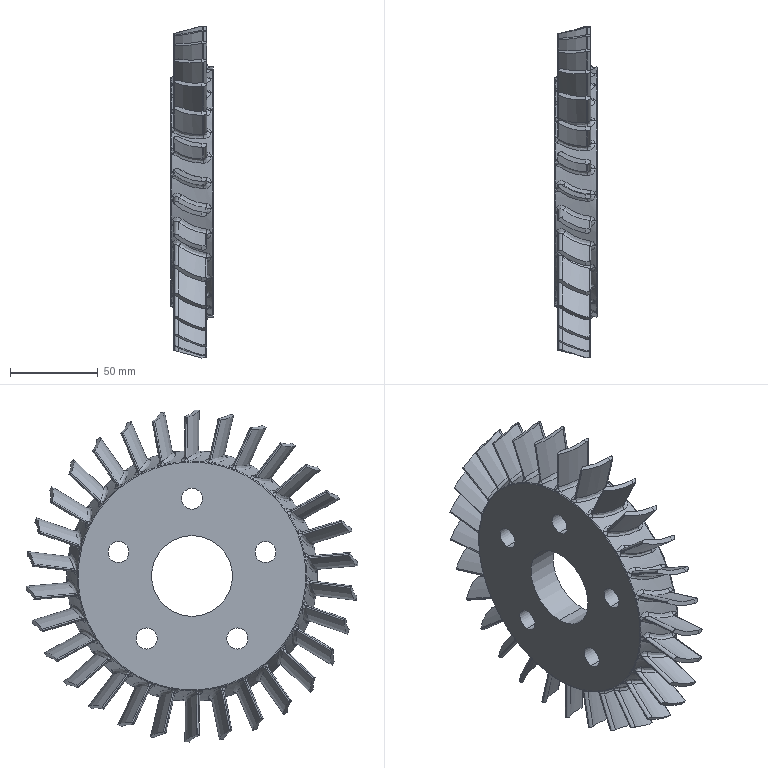Part | STEP file | Previa 01.sldasm-Part-15_Valor predeterminado | 1 solid | 601 faces | box 24.229 x 188.642 x 188.976 mm | volume 257389 mm3 | cylinder 252 | spline 245 | cone 37 | torus 35 | plane 32 | commonest cylinder face diameters 4 x90 1 x60 53.531 x30 58.531 x30 189 x30 12 x10